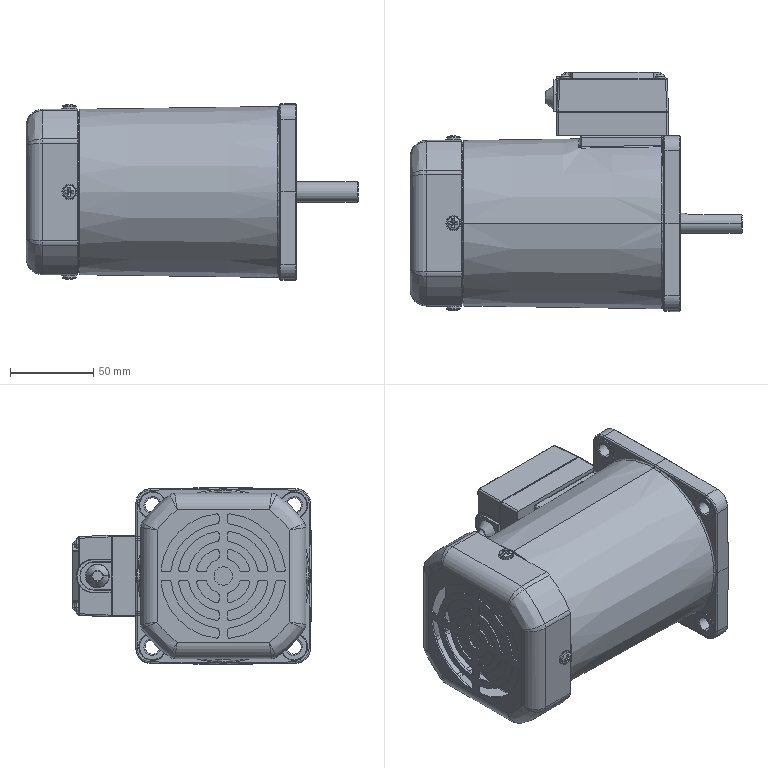Part | STEP file | 200ys04 | 2 solids | 1151 faces | box 199 x 143.386 x 105.972 mm | volume 487784 mm3 | spline 461 | cylinder 345 | plane 299 | cone 38 | torus 8 | commonest cylinder face diameters 0.5 x60 3 x54 4 x42 8 x20 0.4 x16 2 x13